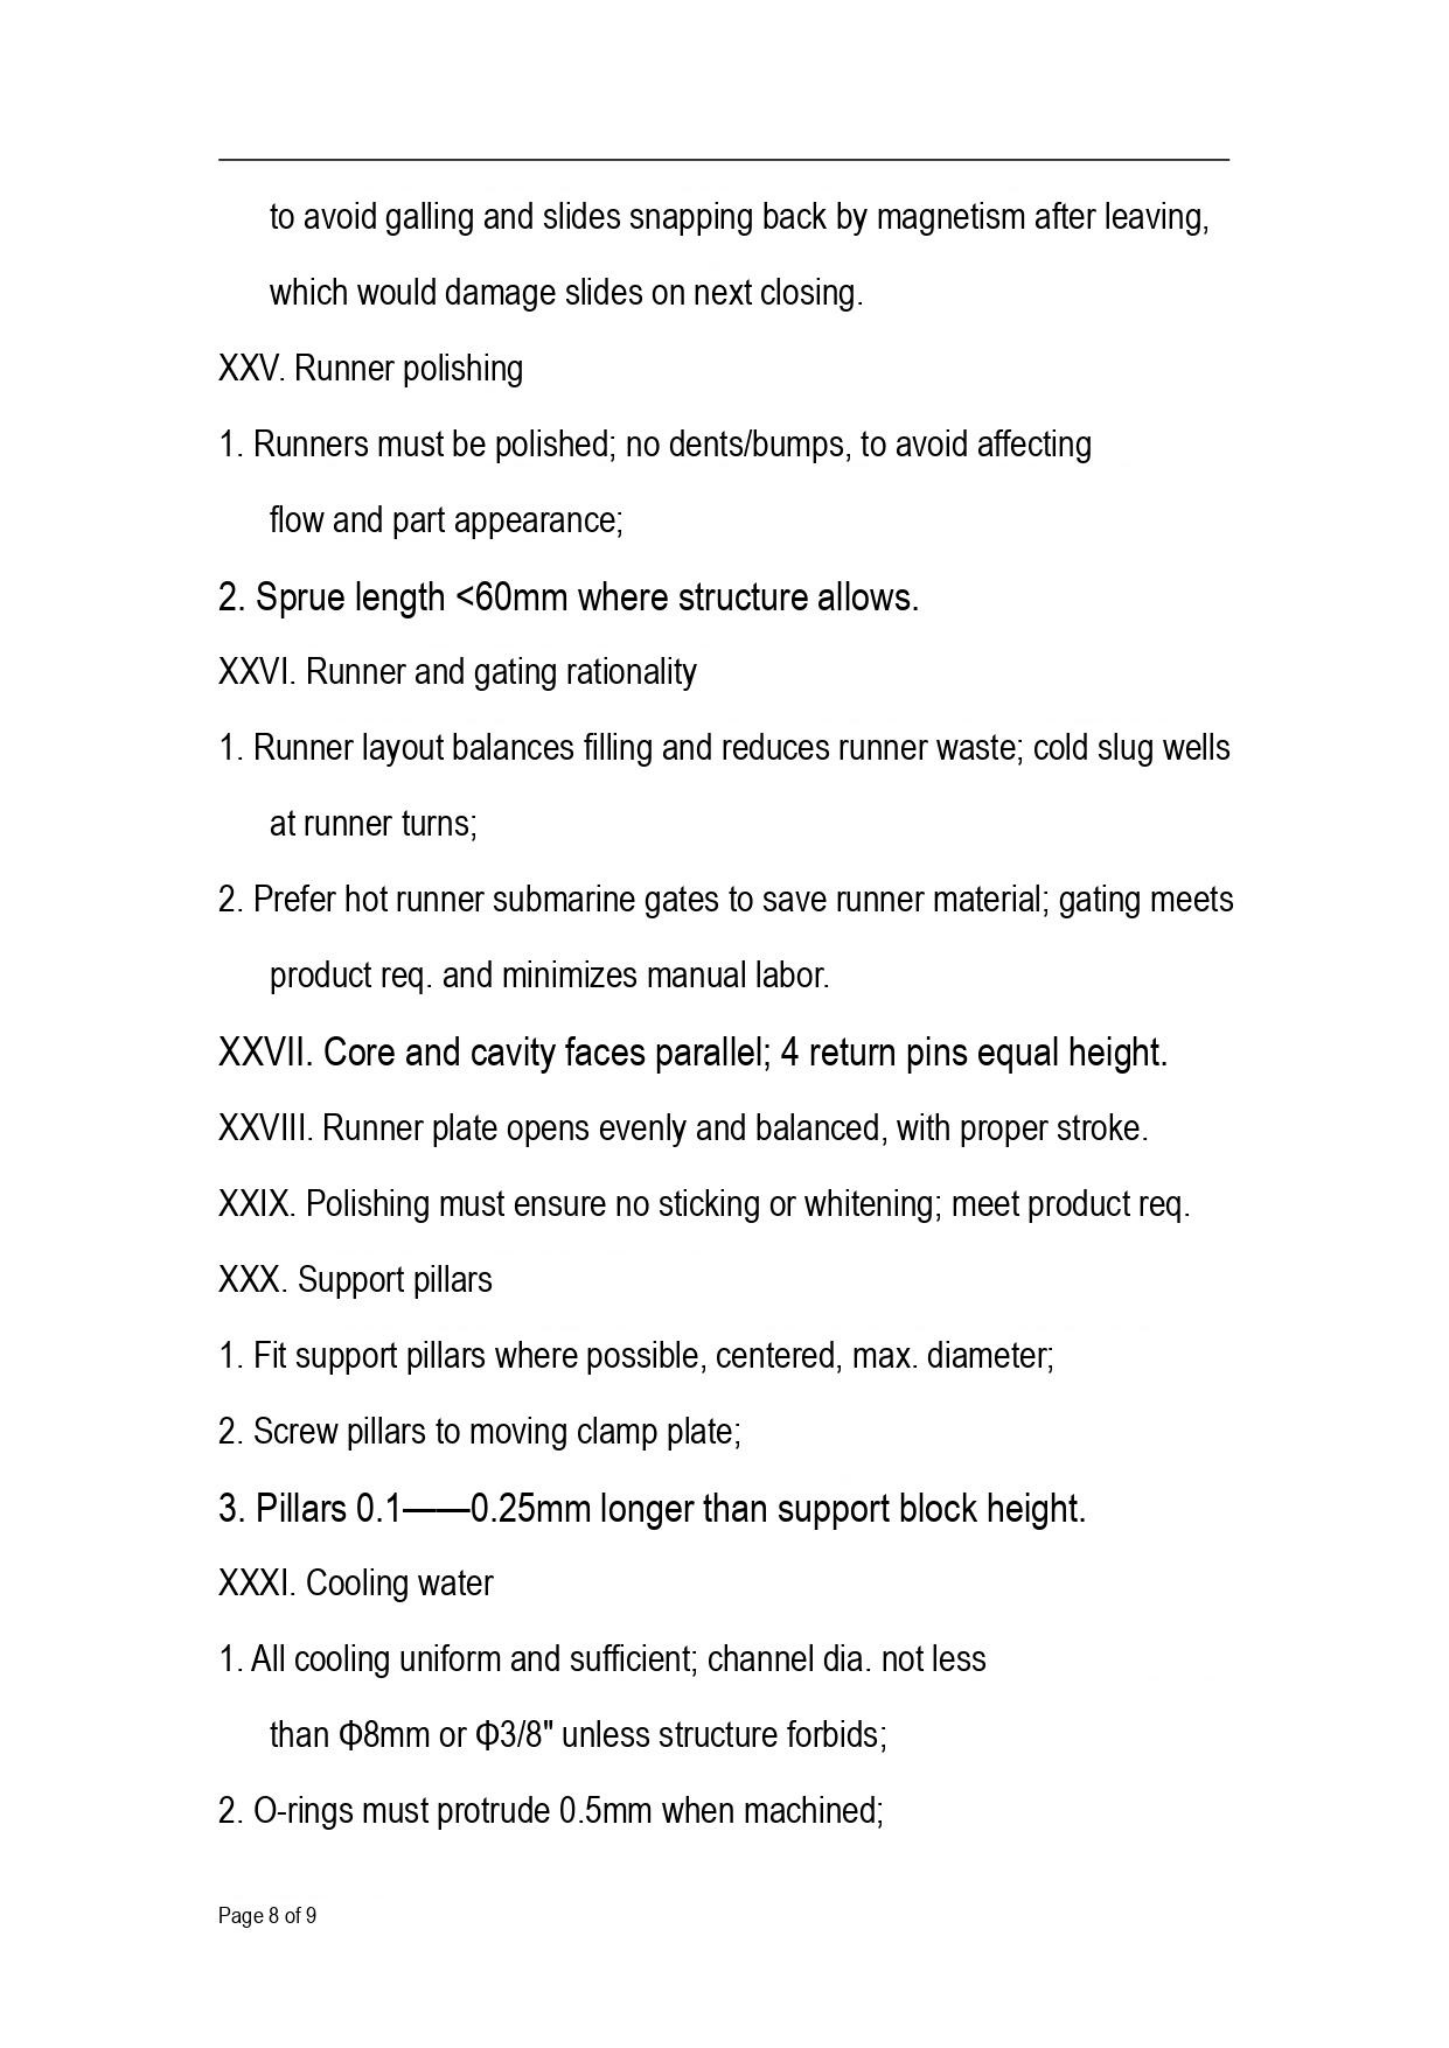to avoid galling and slides snapping back by magnetism after leaving, which would damage slides on next closing.

XXV. Runner polishing

1. Runners must be polished; no dents/bumps, to avoid affecting flow and part appearance;

2. Sprue length <60mm where structure allows.

XXVI. Runner and gating rationality

1. Runner layout balances filling and reduces runner waste; cold slug wells at runner turns;

2. Prefer hot runner submarine gates to save runner material; gating meets product req. and minimizes manual labor.

XXVII. Core and cavity faces parallel; 4 return pins equal height.

XXVIII. Runner plate opens evenly and balanced, with proper stroke.

XXIX. Polishing must ensure no sticking or whitening; meet product req.

XXX. Support pillars

1. Fit support pillars where possible, centered, max. diameter;

2. Screw pillars to moving clamp plate;

3. Pillars 0.1——0.25mm longer than support block height.

XXXI. Cooling water

1. All cooling uniform and sufficient; channel dia. not less than Φ8mm or Φ3/8" unless structure forbids;

2. O-rings must protrude 0.5mm when machined;

Page 8 of 9
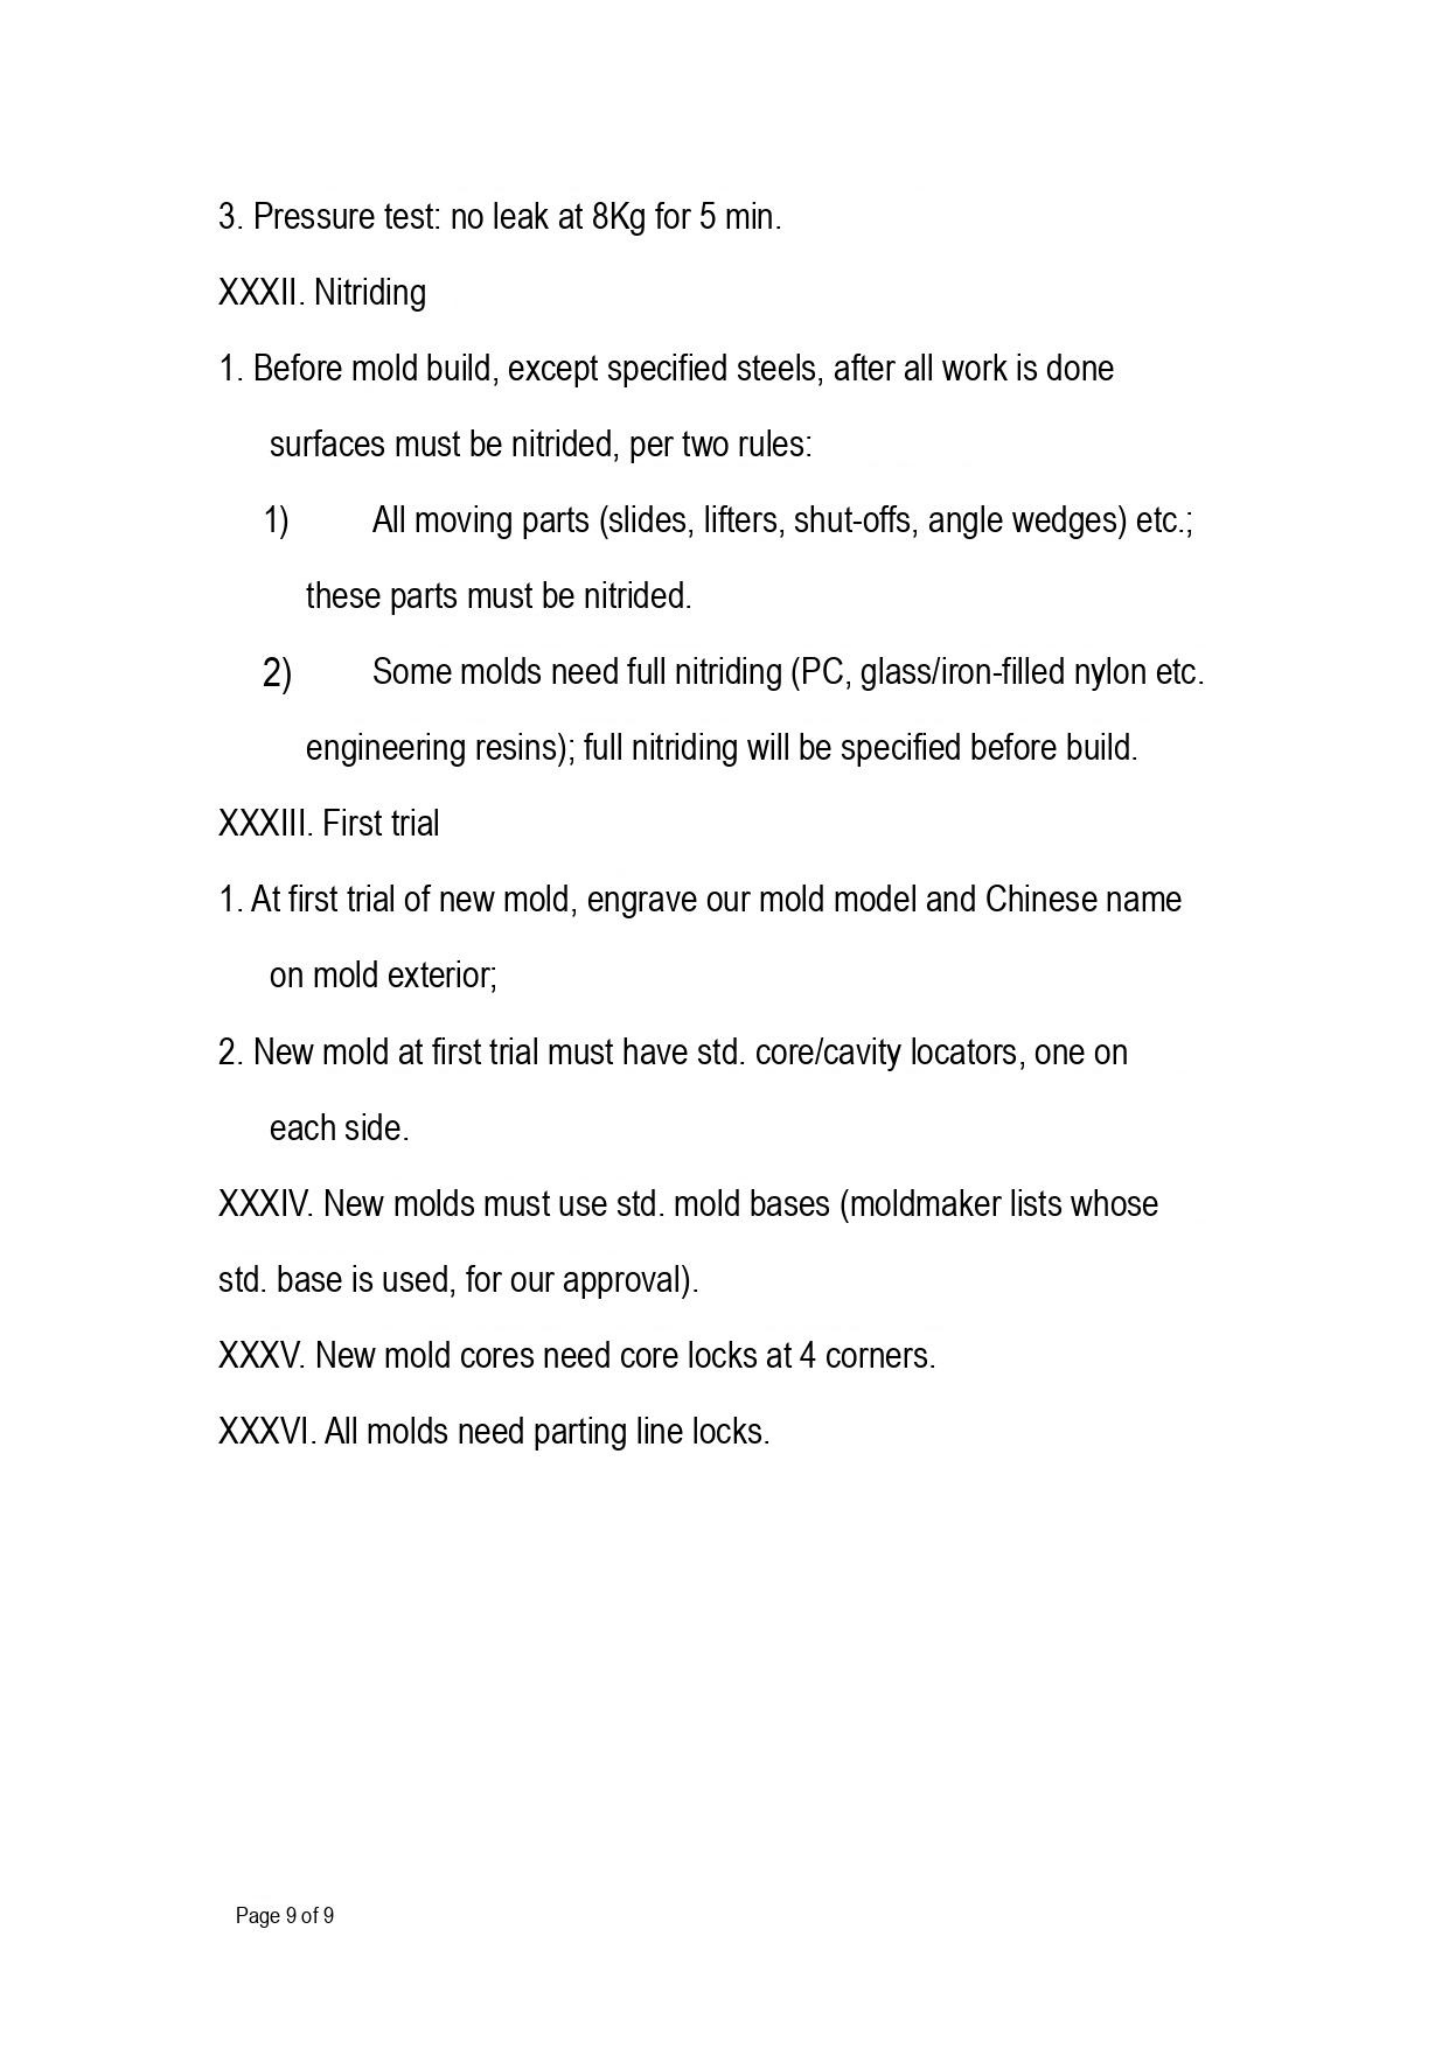3. Pressure test: no leak at 8Kg for 5 min.

XXXII. Nitriding

1. Before mold build, except specified steels, after all work is done surfaces must be nitrided, per two rules:

1) All moving parts (slides, lifters, shut-offs, angle wedges) etc.; these parts must be nitrided.

2) Some molds need full nitriding (PC, glass/iron-filled nylon etc. engineering resins); full nitriding will be specified before build.

XXXIII. First trial

1. At first trial of new mold, engrave our mold model and Chinese name on mold exterior;

2. New mold at first trial must have std. core/cavity locators, one on each side.

XXXIV. New molds must use std. mold bases (moldmaker lists whose std. base is used, for our approval).

XXXV. New mold cores need core locks at 4 corners.

XXXVI. All molds need parting line locks.

Page 9 of 9